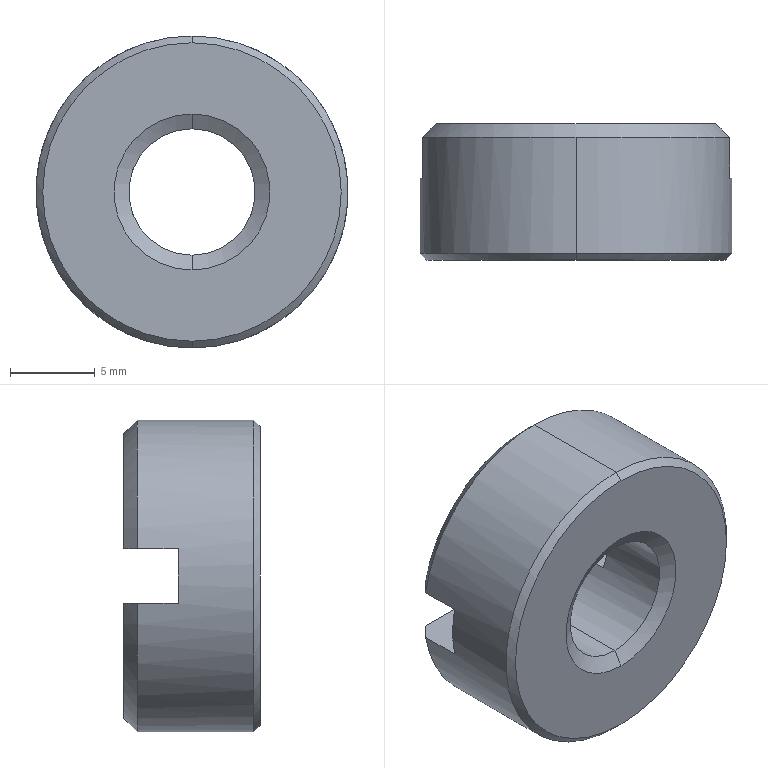Part | SolidWorks | features BaseBody 1 | 1 solid | 19 faces | box 18.462 x 8.077 x 18.462 mm | volume 1664 mm3 | plane 9 | cone 6 | cylinder 4 | commonest cylinder face diameters 7.482 x2 18.462 x2
STEP:
#1=CARTESIAN_POINT('',(66.335,375.615,109.308));
#2=VERTEX_POINT('',#1);
#3=CARTESIAN_POINT('',(57.247,375.615,116.923));
#4=VERTEX_POINT('',#3);
#5=CARTESIAN_POINT('',(57.247,375.615,107.692));
#6=DIRECTION('',(0.,-1.,0.));
#7=DIRECTION('',(0.,0.,-1.));
#8=AXIS2_PLACEMENT_3D('',#5,#6,#7);
#9=CIRCLE('',#8,9.231);
#10=EDGE_CURVE('',#2,#4,#9,.T.);
#11=ORIENTED_EDGE('',*,*,#10,.T.);
#12=CARTESIAN_POINT('',(57.247,368.75,116.923));
#13=VERTEX_POINT('',#12);
#14=CARTESIAN_POINT('',(57.247,376.423,116.923));
#15=DIRECTION('',(0.,-1.,0.));
#16=VECTOR('',#15,1000.);
#17=LINE('',#14,#16);
#18=EDGE_CURVE('',#4,#13,#17,.T.);
#19=ORIENTED_EDGE('',*,*,#18,.T.);
#20=CARTESIAN_POINT('',(57.247,368.75,98.462));
#21=VERTEX_POINT('',#20);
#22=CARTESIAN_POINT('',(57.247,368.75,107.692));
#23=DIRECTION('',(0.,1.,0.));
#24=DIRECTION('',(0.,0.,-1.));
#25=AXIS2_PLACEMENT_3D('',#22,#23,#24);
#26=CIRCLE('',#25,9.231);
#27=EDGE_CURVE('',#13,#21,#26,.T.);
#28=ORIENTED_EDGE('',*,*,#27,.T.);
#29=CARTESIAN_POINT('',(57.247,375.615,98.462));
#30=VERTEX_POINT('',#29);
#31=CARTESIAN_POINT('',(57.247,376.423,98.462));
#32=DIRECTION('',(0.,-1.,0.));
#33=VECTOR('',#32,1000.);
#34=LINE('',#31,#33);
#35=EDGE_CURVE('',#30,#21,#34,.T.);
#36=ORIENTED_EDGE('',*,*,#35,.F.);
#37=CARTESIAN_POINT('',(66.335,375.615,106.077));
#38=VERTEX_POINT('',#37);
#39=CARTESIAN_POINT('',(57.247,375.615,107.692));
#40=DIRECTION('',(0.,-1.,0.));
#41=DIRECTION('',(0.,0.,-1.));
#42=AXIS2_PLACEMENT_3D('',#39,#40,#41);
#43=CIRCLE('',#42,9.231);
#44=EDGE_CURVE('',#30,#38,#43,.T.);
#45=ORIENTED_EDGE('',*,*,#44,.T.);
#46=CARTESIAN_POINT('',(66.335,373.192,106.077));
#47=VERTEX_POINT('',#46);
#48=CARTESIAN_POINT('',(66.335,376.423,106.077));
#49=DIRECTION('',(0.,-1.,0.));
#50=VECTOR('',#49,1000.);
#51=LINE('',#48,#50);
#52=EDGE_CURVE('',#38,#47,#51,.T.);
#53=ORIENTED_EDGE('',*,*,#52,.T.);
#54=CARTESIAN_POINT('',(66.335,373.192,109.308));
#55=VERTEX_POINT('',#54);
#56=CARTESIAN_POINT('',(57.247,373.192,107.692));
#57=DIRECTION('',(0.,-1.,0.));
#58=DIRECTION('',(0.,0.,-1.));
#59=AXIS2_PLACEMENT_3D('',#56,#57,#58);
#60=CIRCLE('',#59,9.231);
#61=EDGE_CURVE('',#47,#55,#60,.T.);
#62=ORIENTED_EDGE('',*,*,#61,.T.);
#63=CARTESIAN_POINT('',(66.335,376.423,109.308));
#64=DIRECTION('',(0.,1.,0.));
#65=VECTOR('',#64,1000.);
#66=LINE('',#63,#65);
#67=EDGE_CURVE('',#55,#2,#66,.T.);
#68=ORIENTED_EDGE('',*,*,#67,.T.);
#69=EDGE_LOOP('',(#11,#19,#28,#36,#45,#53,#62,#68));
#70=FACE_OUTER_BOUND('',#69,.T.);
#71=CARTESIAN_POINT('',(57.247,376.423,107.692));
#72=DIRECTION('',(0.,-1.,0.));
#73=DIRECTION('',(0.,0.,-1.));
#74=AXIS2_PLACEMENT_3D('',#71,#72,#73);
#75=CYLINDRICAL_SURFACE('',#74,9.231);
#76=ADVANCED_FACE('',(#70),#75,.T.);
#77=CARTESIAN_POINT('',(57.247,368.346,116.519));
#78=VERTEX_POINT('',#77);
#79=CARTESIAN_POINT('',(57.247,368.346,98.865));
#80=VERTEX_POINT('',#79);
#81=CARTESIAN_POINT('',(57.247,368.346,107.692));
#82=DIRECTION('',(0.,1.,0.));
#83=DIRECTION('',(0.,0.,1.));
#84=AXIS2_PLACEMENT_3D('',#81,#82,#83);
#85=CIRCLE('',#84,8.827);
#86=EDGE_CURVE('',#78,#80,#85,.T.);
#87=ORIENTED_EDGE('',*,*,#86,.T.);
#88=CARTESIAN_POINT('',(57.247,368.75,98.462));
#89=DIRECTION('',(0.,0.7071,-0.7071));
#90=VECTOR('',#89,1000.);
#91=LINE('',#88,#90);
#92=EDGE_CURVE('',#80,#21,#91,.T.);
#93=ORIENTED_EDGE('',*,*,#92,.T.);
#94=ORIENTED_EDGE('',*,*,#27,.F.);
#95=CARTESIAN_POINT('',(57.247,368.75,116.923));
#96=DIRECTION('',(0.,0.7071,0.7071));
#97=VECTOR('',#96,1000.);
#98=LINE('',#95,#97);
#99=EDGE_CURVE('',#78,#13,#98,.T.);
#100=ORIENTED_EDGE('',*,*,#99,.F.);
#101=EDGE_LOOP('',(#87,#93,#94,#100));
#102=FACE_OUTER_BOUND('',#101,.T.);
#103=CARTESIAN_POINT('',(57.247,368.75,107.692));
#104=DIRECTION('',(0.,1.,0.));
#105=DIRECTION('',(0.,0.,1.));
#106=AXIS2_PLACEMENT_3D('',#103,#104,#105);
#107=CONICAL_SURFACE('',#106,9.231,0.7854);
#108=ADVANCED_FACE('',(#102),#107,.T.);
#109=CARTESIAN_POINT('',(57.247,376.423,111.433));
#110=VERTEX_POINT('',#109);
#111=CARTESIAN_POINT('',(53.873,376.423,109.308));
#112=VERTEX_POINT('',#111);
#113=CARTESIAN_POINT('',(57.247,376.423,107.692));
#114=DIRECTION('',(0.,-1.,0.));
#115=DIRECTION('',(0.,0.,-1.));
#116=AXIS2_PLACEMENT_3D('',#113,#114,#115);
#117=CIRCLE('',#116,3.741);
#118=EDGE_CURVE('',#110,#112,#117,.T.);
#119=ORIENTED_EDGE('',*,*,#118,.F.);
#120=CARTESIAN_POINT('',(57.247,368.851,111.433));
#121=VERTEX_POINT('',#120);
#122=CARTESIAN_POINT('',(57.247,376.423,111.433));
#123=DIRECTION('',(0.,-1.,0.));
#124=VECTOR('',#123,1000.);
#125=LINE('',#122,#124);
#126=EDGE_CURVE('',#110,#121,#125,.T.);
#127=ORIENTED_EDGE('',*,*,#126,.T.);
#128=CARTESIAN_POINT('',(57.247,368.851,103.952));
#129=VERTEX_POINT('',#128);
#130=CARTESIAN_POINT('',(57.247,368.851,107.692));
#131=DIRECTION('',(0.,1.,0.));
#132=DIRECTION('',(0.,0.,-1.));
#133=AXIS2_PLACEMENT_3D('',#130,#131,#132);
#134=CIRCLE('',#133,3.741);
#135=EDGE_CURVE('',#129,#121,#134,.T.);
#136=ORIENTED_EDGE('',*,*,#135,.F.);
#137=CARTESIAN_POINT('',(57.247,376.423,103.952));
#138=VERTEX_POINT('',#137);
#139=CARTESIAN_POINT('',(57.247,376.423,103.952));
#140=DIRECTION('',(0.,-1.,0.));
#141=VECTOR('',#140,1000.);
#142=LINE('',#139,#141);
#143=EDGE_CURVE('',#138,#129,#142,.T.);
#144=ORIENTED_EDGE('',*,*,#143,.F.);
#145=CARTESIAN_POINT('',(53.873,376.423,106.077));
#146=VERTEX_POINT('',#145);
#147=CARTESIAN_POINT('',(57.247,376.423,107.692));
#148=DIRECTION('',(0.,1.,0.));
#149=DIRECTION('',(0.,0.,-1.));
#150=AXIS2_PLACEMENT_3D('',#147,#148,#149);
#151=CIRCLE('',#150,3.741);
#152=EDGE_CURVE('',#138,#146,#151,.T.);
#153=ORIENTED_EDGE('',*,*,#152,.T.);
#154=CARTESIAN_POINT('',(53.873,373.192,106.077));
#155=VERTEX_POINT('',#154);
#156=CARTESIAN_POINT('',(53.873,381.269,106.077));
#157=DIRECTION('',(0.,1.,0.));
#158=VECTOR('',#157,1000.);
#159=LINE('',#156,#158);
#160=EDGE_CURVE('',#155,#146,#159,.T.);
#161=ORIENTED_EDGE('',*,*,#160,.F.);
#162=CARTESIAN_POINT('',(53.873,373.192,109.308));
#163=VERTEX_POINT('',#162);
#164=CARTESIAN_POINT('',(57.247,373.192,107.692));
#165=DIRECTION('',(0.,-1.,0.));
#166=DIRECTION('',(0.,0.,-1.));
#167=AXIS2_PLACEMENT_3D('',#164,#165,#166);
#168=CIRCLE('',#167,3.741);
#169=EDGE_CURVE('',#163,#155,#168,.T.);
#170=ORIENTED_EDGE('',*,*,#169,.F.);
#171=CARTESIAN_POINT('',(53.873,373.192,109.308));
#172=DIRECTION('',(0.,-1.,0.));
#173=VECTOR('',#172,1000.);
#174=LINE('',#171,#173);
#175=EDGE_CURVE('',#112,#163,#174,.T.);
#176=ORIENTED_EDGE('',*,*,#175,.F.);
#177=EDGE_LOOP('',(#119,#127,#136,#144,#153,#161,#170,#176));
#178=FACE_OUTER_BOUND('',#177,.T.);
#179=CARTESIAN_POINT('',(57.247,376.423,107.692));
#180=DIRECTION('',(0.,-1.,0.));
#181=DIRECTION('',(0.,0.,-1.));
#182=AXIS2_PLACEMENT_3D('',#179,#180,#181);
#183=CYLINDRICAL_SURFACE('',#182,3.741);
#184=ADVANCED_FACE('',(#178),#183,.F.);
#185=ORIENTED_EDGE('',*,*,#135,.T.);
#186=CARTESIAN_POINT('',(57.247,368.346,112.308));
#187=VERTEX_POINT('',#186);
#188=CARTESIAN_POINT('',(57.247,368.346,112.308));
#189=DIRECTION('',(0.,-0.5,0.866));
#190=VECTOR('',#189,1000.);
#191=LINE('',#188,#190);
#192=EDGE_CURVE('',#121,#187,#191,.T.);
#193=ORIENTED_EDGE('',*,*,#192,.T.);
#194=CARTESIAN_POINT('',(57.247,368.346,103.077));
#195=VERTEX_POINT('',#194);
#196=CARTESIAN_POINT('',(57.247,368.346,107.692));
#197=DIRECTION('',(0.,-1.,0.));
#198=DIRECTION('',(0.,0.,-1.));
#199=AXIS2_PLACEMENT_3D('',#196,#197,#198);
#200=CIRCLE('',#199,4.615);
#201=EDGE_CURVE('',#187,#195,#200,.T.);
#202=ORIENTED_EDGE('',*,*,#201,.T.);
#203=CARTESIAN_POINT('',(57.247,368.346,103.077));
#204=DIRECTION('',(0.,-0.5,-0.866));
#205=VECTOR('',#204,1000.);
#206=LINE('',#203,#205);
#207=EDGE_CURVE('',#129,#195,#206,.T.);
#208=ORIENTED_EDGE('',*,*,#207,.F.);
#209=EDGE_LOOP('',(#185,#193,#202,#208));
#210=FACE_OUTER_BOUND('',#209,.T.);
#211=CARTESIAN_POINT('',(57.247,368.346,107.692));
#212=DIRECTION('',(0.,-1.,0.));
#213=DIRECTION('',(0.,0.,-1.));
#214=AXIS2_PLACEMENT_3D('',#211,#212,#213);
#215=CONICAL_SURFACE('',#214,4.615,1.047);
#216=ADVANCED_FACE('',(#210),#215,.F.);
#217=ORIENTED_EDGE('',*,*,#18,.F.);
#218=CARTESIAN_POINT('',(48.158,375.615,109.308));
#219=VERTEX_POINT('',#218);
#220=CARTESIAN_POINT('',(57.247,375.615,107.692));
#221=DIRECTION('',(0.,-1.,0.));
#222=DIRECTION('',(0.,0.,-1.));
#223=AXIS2_PLACEMENT_3D('',#220,#221,#222);
#224=CIRCLE('',#223,9.231);
#225=EDGE_CURVE('',#4,#219,#224,.T.);
#226=ORIENTED_EDGE('',*,*,#225,.T.);
#227=CARTESIAN_POINT('',(48.158,373.192,109.308));
#228=VERTEX_POINT('',#227);
#229=CARTESIAN_POINT('',(48.158,376.423,109.308));
#230=DIRECTION('',(0.,-1.,0.));
#231=VECTOR('',#230,1000.);
#232=LINE('',#229,#231);
#233=EDGE_CURVE('',#219,#228,#232,.T.);
#234=ORIENTED_EDGE('',*,*,#233,.T.);
#235=CARTESIAN_POINT('',(48.158,373.192,106.077));
#236=VERTEX_POINT('',#235);
#237=CARTESIAN_POINT('',(57.247,373.192,107.692));
#238=DIRECTION('',(0.,-1.,0.));
#239=DIRECTION('',(0.,0.,-1.));
#240=AXIS2_PLACEMENT_3D('',#237,#238,#239);
#241=CIRCLE('',#240,9.231);
#242=EDGE_CURVE('',#228,#236,#241,.T.);
#243=ORIENTED_EDGE('',*,*,#242,.T.);
#244=CARTESIAN_POINT('',(48.158,375.615,106.077));
#245=VERTEX_POINT('',#244);
#246=CARTESIAN_POINT('',(48.158,376.423,106.077));
#247=DIRECTION('',(0.,1.,0.));
#248=VECTOR('',#247,1000.);
#249=LINE('',#246,#248);
#250=EDGE_CURVE('',#236,#245,#249,.T.);
#251=ORIENTED_EDGE('',*,*,#250,.T.);
#252=CARTESIAN_POINT('',(57.247,375.615,107.692));
#253=DIRECTION('',(0.,-1.,0.));
#254=DIRECTION('',(0.,0.,-1.));
#255=AXIS2_PLACEMENT_3D('',#252,#253,#254);
#256=CIRCLE('',#255,9.231);
#257=EDGE_CURVE('',#245,#30,#256,.T.);
#258=ORIENTED_EDGE('',*,*,#257,.T.);
#259=ORIENTED_EDGE('',*,*,#35,.T.);
#260=CARTESIAN_POINT('',(57.247,368.75,107.692));
#261=DIRECTION('',(0.,1.,0.));
#262=DIRECTION('',(0.,0.,-1.));
#263=AXIS2_PLACEMENT_3D('',#260,#261,#262);
#264=CIRCLE('',#263,9.231);
#265=EDGE_CURVE('',#21,#13,#264,.T.);
#266=ORIENTED_EDGE('',*,*,#265,.T.);
#267=EDGE_LOOP('',(#217,#226,#234,#243,#251,#258,#259,#266));
#268=FACE_OUTER_BOUND('',#267,.T.);
#269=CARTESIAN_POINT('',(57.247,376.423,107.692));
#270=DIRECTION('',(0.,-1.,0.));
#271=DIRECTION('',(0.,0.,-1.));
#272=AXIS2_PLACEMENT_3D('',#269,#270,#271);
#273=CYLINDRICAL_SURFACE('',#272,9.231);
#274=ADVANCED_FACE('',(#268),#273,.T.);
#275=ORIENTED_EDGE('',*,*,#257,.F.);
#276=CARTESIAN_POINT('',(48.98,376.423,106.077));
#277=VERTEX_POINT('',#276);
#278=CARTESIAN_POINT('',(48.158,375.615,106.077));
#279=CARTESIAN_POINT('',(48.432,375.885,106.077));
#280=CARTESIAN_POINT('',(48.706,376.154,106.077));
#281=CARTESIAN_POINT('',(48.98,376.423,106.077));
#282=B_SPLINE_CURVE_WITH_KNOTS('',3,(#278,#279,#280,#281),.UNSPECIFIED.,.F.,.F.,(4,4),(0.,0.001152),.UNSPECIFIED.);
#283=EDGE_CURVE('',#245,#277,#282,.T.);
#284=ORIENTED_EDGE('',*,*,#283,.T.);
#285=CARTESIAN_POINT('',(65.513,376.423,106.077));
#286=VERTEX_POINT('',#285);
#287=CARTESIAN_POINT('',(57.247,376.423,107.692));
#288=DIRECTION('',(0.,-1.,0.));
#289=DIRECTION('',(1.,0.,0.));
#290=AXIS2_PLACEMENT_3D('',#287,#288,#289);
#291=CIRCLE('',#290,8.423);
#292=EDGE_CURVE('',#277,#286,#291,.T.);
#293=ORIENTED_EDGE('',*,*,#292,.T.);
#294=CARTESIAN_POINT('',(65.513,376.423,106.077));
#295=CARTESIAN_POINT('',(65.787,376.154,106.077));
#296=CARTESIAN_POINT('',(66.061,375.885,106.077));
#297=CARTESIAN_POINT('',(66.335,375.615,106.077));
#298=B_SPLINE_CURVE_WITH_KNOTS('',3,(#294,#295,#296,#297),.UNSPECIFIED.,.F.,.F.,(4,4),(0.,0.001152),.UNSPECIFIED.);
#299=EDGE_CURVE('',#286,#38,#298,.T.);
#300=ORIENTED_EDGE('',*,*,#299,.T.);
#301=ORIENTED_EDGE('',*,*,#44,.F.);
#302=EDGE_LOOP('',(#275,#284,#293,#300,#301));
#303=FACE_OUTER_BOUND('',#302,.T.);
#304=CARTESIAN_POINT('',(57.247,375.615,107.692));
#305=DIRECTION('',(0.,-1.,0.));
#306=DIRECTION('',(1.,0.,0.));
#307=AXIS2_PLACEMENT_3D('',#304,#305,#306);
#308=CONICAL_SURFACE('',#307,9.231,0.7854);
#309=ADVANCED_FACE('',(#303),#308,.T.);
#310=ORIENTED_EDGE('',*,*,#160,.T.);
#311=CARTESIAN_POINT('',(38.785,376.423,106.077));
#312=DIRECTION('',(-1.,0.,0.));
#313=VECTOR('',#312,1000.);
#314=LINE('',#311,#313);
#315=EDGE_CURVE('',#146,#277,#314,.T.);
#316=ORIENTED_EDGE('',*,*,#315,.T.);
#317=ORIENTED_EDGE('',*,*,#283,.F.);
#318=ORIENTED_EDGE('',*,*,#250,.F.);
#319=CARTESIAN_POINT('',(38.785,373.192,106.077));
#320=DIRECTION('',(1.,0.,0.));
#321=VECTOR('',#320,1000.);
#322=LINE('',#319,#321);
#323=EDGE_CURVE('',#236,#155,#322,.T.);
#324=ORIENTED_EDGE('',*,*,#323,.T.);
#325=EDGE_LOOP('',(#310,#316,#317,#318,#324));
#326=FACE_OUTER_BOUND('',#325,.T.);
#327=CARTESIAN_POINT('',(38.785,381.269,106.077));
#328=DIRECTION('',(0.,0.,1.));
#329=DIRECTION('',(1.,0.,0.));
#330=AXIS2_PLACEMENT_3D('',#327,#328,#329);
#331=PLANE('',#330);
#332=ADVANCED_FACE('',(#326),#331,.T.);
#333=CARTESIAN_POINT('',(38.785,373.192,109.308));
#334=DIRECTION('',(1.,0.,0.));
#335=VECTOR('',#334,1000.);
#336=LINE('',#333,#335);
#337=EDGE_CURVE('',#228,#163,#336,.T.);
#338=ORIENTED_EDGE('',*,*,#337,.T.);
#339=ORIENTED_EDGE('',*,*,#169,.T.);
#340=ORIENTED_EDGE('',*,*,#323,.F.);
#341=ORIENTED_EDGE('',*,*,#242,.F.);
#342=EDGE_LOOP('',(#338,#339,#340,#341));
#343=FACE_OUTER_BOUND('',#342,.T.);
#344=CARTESIAN_POINT('',(38.785,373.192,106.077));
#345=DIRECTION('',(0.,1.,0.));
#346=DIRECTION('',(0.,0.,1.));
#347=AXIS2_PLACEMENT_3D('',#344,#345,#346);
#348=PLANE('',#347);
#349=ADVANCED_FACE('',(#343),#348,.T.);
#350=CARTESIAN_POINT('',(48.98,376.423,109.308));
#351=VERTEX_POINT('',#350);
#352=CARTESIAN_POINT('',(38.785,376.423,109.308));
#353=DIRECTION('',(1.,0.,0.));
#354=VECTOR('',#353,1000.);
#355=LINE('',#352,#354);
#356=EDGE_CURVE('',#351,#112,#355,.T.);
#357=ORIENTED_EDGE('',*,*,#356,.T.);
#358=ORIENTED_EDGE('',*,*,#175,.T.);
#359=ORIENTED_EDGE('',*,*,#337,.F.);
#360=ORIENTED_EDGE('',*,*,#233,.F.);
#361=CARTESIAN_POINT('',(48.158,375.615,109.308));
#362=CARTESIAN_POINT('',(48.432,375.885,109.308));
#363=CARTESIAN_POINT('',(48.706,376.154,109.308));
#364=CARTESIAN_POINT('',(48.98,376.423,109.308));
#365=B_SPLINE_CURVE_WITH_KNOTS('',3,(#361,#362,#363,#364),.UNSPECIFIED.,.F.,.F.,(4,4),(0.,0.001152),.UNSPECIFIED.);
#366=EDGE_CURVE('',#219,#351,#365,.T.);
#367=ORIENTED_EDGE('',*,*,#366,.T.);
#368=EDGE_LOOP('',(#357,#358,#359,#360,#367));
#369=FACE_OUTER_BOUND('',#368,.T.);
#370=CARTESIAN_POINT('',(38.785,373.192,109.308));
#371=DIRECTION('',(0.,0.,-1.));
#372=DIRECTION('',(-1.,0.,0.));
#373=AXIS2_PLACEMENT_3D('',#370,#371,#372);
#374=PLANE('',#373);
#375=ADVANCED_FACE('',(#369),#374,.T.);
#376=ORIENTED_EDGE('',*,*,#10,.F.);
#377=CARTESIAN_POINT('',(65.513,376.423,109.308));
#378=VERTEX_POINT('',#377);
#379=CARTESIAN_POINT('',(66.335,375.615,109.308));
#380=CARTESIAN_POINT('',(66.061,375.885,109.308));
#381=CARTESIAN_POINT('',(65.787,376.154,109.308));
#382=CARTESIAN_POINT('',(65.513,376.423,109.308));
#383=B_SPLINE_CURVE_WITH_KNOTS('',3,(#379,#380,#381,#382),.UNSPECIFIED.,.F.,.F.,(4,4),(0.,0.001152),.UNSPECIFIED.);
#384=EDGE_CURVE('',#2,#378,#383,.T.);
#385=ORIENTED_EDGE('',*,*,#384,.T.);
#386=CARTESIAN_POINT('',(57.247,376.423,107.692));
#387=DIRECTION('',(0.,-1.,0.));
#388=DIRECTION('',(0.,0.,-1.));
#389=AXIS2_PLACEMENT_3D('',#386,#387,#388);
#390=CIRCLE('',#389,8.423);
#391=EDGE_CURVE('',#378,#351,#390,.T.);
#392=ORIENTED_EDGE('',*,*,#391,.T.);
#393=ORIENTED_EDGE('',*,*,#366,.F.);
#394=ORIENTED_EDGE('',*,*,#225,.F.);
#395=EDGE_LOOP('',(#376,#385,#392,#393,#394));
#396=FACE_OUTER_BOUND('',#395,.T.);
#397=CARTESIAN_POINT('',(57.247,375.615,107.692));
#398=DIRECTION('',(0.,-1.,0.));
#399=DIRECTION('',(0.,0.,-1.));
#400=AXIS2_PLACEMENT_3D('',#397,#398,#399);
#401=CONICAL_SURFACE('',#400,9.231,0.7854);
#402=ADVANCED_FACE('',(#396),#401,.T.);
#403=ORIENTED_EDGE('',*,*,#92,.F.);
#404=CARTESIAN_POINT('',(57.247,368.346,107.692));
#405=DIRECTION('',(0.,1.,0.));
#406=DIRECTION('',(0.,0.,1.));
#407=AXIS2_PLACEMENT_3D('',#404,#405,#406);
#408=CIRCLE('',#407,8.827);
#409=EDGE_CURVE('',#80,#78,#408,.T.);
#410=ORIENTED_EDGE('',*,*,#409,.T.);
#411=ORIENTED_EDGE('',*,*,#99,.T.);
#412=ORIENTED_EDGE('',*,*,#265,.F.);
#413=EDGE_LOOP('',(#403,#410,#411,#412));
#414=FACE_OUTER_BOUND('',#413,.T.);
#415=CARTESIAN_POINT('',(57.247,368.75,107.692));
#416=DIRECTION('',(0.,1.,0.));
#417=DIRECTION('',(0.,0.,1.));
#418=AXIS2_PLACEMENT_3D('',#415,#416,#417);
#419=CONICAL_SURFACE('',#418,9.231,0.7854);
#420=ADVANCED_FACE('',(#414),#419,.T.);
#421=CARTESIAN_POINT('',(60.621,376.423,106.077));
#422=VERTEX_POINT('',#421);
#423=CARTESIAN_POINT('',(38.785,376.423,106.077));
#424=DIRECTION('',(-1.,0.,0.));
#425=VECTOR('',#424,1000.);
#426=LINE('',#423,#425);
#427=EDGE_CURVE('',#286,#422,#426,.T.);
#428=ORIENTED_EDGE('',*,*,#427,.T.);
#429=CARTESIAN_POINT('',(60.621,373.192,106.077));
#430=VERTEX_POINT('',#429);
#431=CARTESIAN_POINT('',(60.621,381.269,106.077));
#432=DIRECTION('',(0.,-1.,0.));
#433=VECTOR('',#432,1000.);
#434=LINE('',#431,#433);
#435=EDGE_CURVE('',#422,#430,#434,.T.);
#436=ORIENTED_EDGE('',*,*,#435,.T.);
#437=CARTESIAN_POINT('',(38.785,373.192,106.077));
#438=DIRECTION('',(1.,0.,0.));
#439=VECTOR('',#438,1000.);
#440=LINE('',#437,#439);
#441=EDGE_CURVE('',#430,#47,#440,.T.);
#442=ORIENTED_EDGE('',*,*,#441,.T.);
#443=ORIENTED_EDGE('',*,*,#52,.F.);
#444=ORIENTED_EDGE('',*,*,#299,.F.);
#445=EDGE_LOOP('',(#428,#436,#442,#443,#444));
#446=FACE_OUTER_BOUND('',#445,.T.);
#447=CARTESIAN_POINT('',(38.785,381.269,106.077));
#448=DIRECTION('',(0.,0.,1.));
#449=DIRECTION('',(1.,0.,0.));
#450=AXIS2_PLACEMENT_3D('',#447,#448,#449);
#451=PLANE('',#450);
#452=ADVANCED_FACE('',(#446),#451,.T.);
#453=ORIENTED_EDGE('',*,*,#315,.F.);
#454=ORIENTED_EDGE('',*,*,#152,.F.);
#455=CARTESIAN_POINT('',(57.247,376.423,107.692));
#456=DIRECTION('',(0.,1.,0.));
#457=DIRECTION('',(0.,0.,-1.));
#458=AXIS2_PLACEMENT_3D('',#455,#456,#457);
#459=CIRCLE('',#458,3.741);
#460=EDGE_CURVE('',#422,#138,#459,.T.);
#461=ORIENTED_EDGE('',*,*,#460,.F.);
#462=ORIENTED_EDGE('',*,*,#427,.F.);
#463=ORIENTED_EDGE('',*,*,#292,.F.);
#464=EDGE_LOOP('',(#453,#454,#461,#462,#463));
#465=FACE_OUTER_BOUND('',#464,.T.);
#466=CARTESIAN_POINT('',(48.823,376.423,107.692));
#467=DIRECTION('',(0.,-1.,0.));
#468=DIRECTION('',(0.,0.,-1.));
#469=AXIS2_PLACEMENT_3D('',#466,#467,#468);
#470=PLANE('',#469);
#471=ADVANCED_FACE('',(#465),#470,.F.);
#472=ORIENTED_EDGE('',*,*,#126,.F.);
#473=CARTESIAN_POINT('',(60.621,376.423,109.308));
#474=VERTEX_POINT('',#473);
#475=CARTESIAN_POINT('',(57.247,376.423,107.692));
#476=DIRECTION('',(0.,-1.,0.));
#477=DIRECTION('',(0.,0.,-1.));
#478=AXIS2_PLACEMENT_3D('',#475,#476,#477);
#479=CIRCLE('',#478,3.741);
#480=EDGE_CURVE('',#474,#110,#479,.T.);
#481=ORIENTED_EDGE('',*,*,#480,.F.);
#482=CARTESIAN_POINT('',(60.621,373.192,109.308));
#483=VERTEX_POINT('',#482);
#484=CARTESIAN_POINT('',(60.621,373.192,109.308));
#485=DIRECTION('',(0.,1.,0.));
#486=VECTOR('',#485,1000.);
#487=LINE('',#484,#486);
#488=EDGE_CURVE('',#483,#474,#487,.T.);
#489=ORIENTED_EDGE('',*,*,#488,.F.);
#490=CARTESIAN_POINT('',(57.247,373.192,107.692));
#491=DIRECTION('',(0.,-1.,0.));
#492=DIRECTION('',(0.,0.,-1.));
#493=AXIS2_PLACEMENT_3D('',#490,#491,#492);
#494=CIRCLE('',#493,3.741);
#495=EDGE_CURVE('',#430,#483,#494,.T.);
#496=ORIENTED_EDGE('',*,*,#495,.F.);
#497=ORIENTED_EDGE('',*,*,#435,.F.);
#498=ORIENTED_EDGE('',*,*,#460,.T.);
#499=ORIENTED_EDGE('',*,*,#143,.T.);
#500=CARTESIAN_POINT('',(57.247,368.851,107.692));
#501=DIRECTION('',(0.,1.,0.));
#502=DIRECTION('',(0.,0.,-1.));
#503=AXIS2_PLACEMENT_3D('',#500,#501,#502);
#504=CIRCLE('',#503,3.741);
#505=EDGE_CURVE('',#121,#129,#504,.T.);
#506=ORIENTED_EDGE('',*,*,#505,.F.);
#507=EDGE_LOOP('',(#472,#481,#489,#496,#497,#498,#499,#506));
#508=FACE_OUTER_BOUND('',#507,.T.);
#509=CARTESIAN_POINT('',(57.247,376.423,107.692));
#510=DIRECTION('',(0.,-1.,0.));
#511=DIRECTION('',(0.,0.,-1.));
#512=AXIS2_PLACEMENT_3D('',#509,#510,#511);
#513=CYLINDRICAL_SURFACE('',#512,3.741);
#514=ADVANCED_FACE('',(#508),#513,.F.);
#515=CARTESIAN_POINT('',(48.823,376.423,109.308));
#516=DIRECTION('',(1.,0.,0.));
#517=VECTOR('',#516,1000.);
#518=LINE('',#515,#517);
#519=EDGE_CURVE('',#474,#378,#518,.T.);
#520=ORIENTED_EDGE('',*,*,#519,.F.);
#521=ORIENTED_EDGE('',*,*,#480,.T.);
#522=ORIENTED_EDGE('',*,*,#118,.T.);
#523=ORIENTED_EDGE('',*,*,#356,.F.);
#524=ORIENTED_EDGE('',*,*,#391,.F.);
#525=EDGE_LOOP('',(#520,#521,#522,#523,#524));
#526=FACE_OUTER_BOUND('',#525,.T.);
#527=CARTESIAN_POINT('',(48.823,376.423,107.692));
#528=DIRECTION('',(0.,-1.,0.));
#529=DIRECTION('',(0.,0.,-1.));
#530=AXIS2_PLACEMENT_3D('',#527,#528,#529);
#531=PLANE('',#530);
#532=ADVANCED_FACE('',(#526),#531,.F.);
#533=ORIENTED_EDGE('',*,*,#488,.T.);
#534=ORIENTED_EDGE('',*,*,#519,.T.);
#535=ORIENTED_EDGE('',*,*,#384,.F.);
#536=ORIENTED_EDGE('',*,*,#67,.F.);
#537=CARTESIAN_POINT('',(38.785,373.192,109.308));
#538=DIRECTION('',(-1.,0.,0.));
#539=VECTOR('',#538,1000.);
#540=LINE('',#537,#539);
#541=EDGE_CURVE('',#55,#483,#540,.T.);
#542=ORIENTED_EDGE('',*,*,#541,.T.);
#543=EDGE_LOOP('',(#533,#534,#535,#536,#542));
#544=FACE_OUTER_BOUND('',#543,.T.);
#545=CARTESIAN_POINT('',(38.785,373.192,109.308));
#546=DIRECTION('',(0.,0.,-1.));
#547=DIRECTION('',(-1.,0.,0.));
#548=AXIS2_PLACEMENT_3D('',#545,#546,#547);
#549=PLANE('',#548);
#550=ADVANCED_FACE('',(#544),#549,.T.);
#551=ORIENTED_EDGE('',*,*,#441,.F.);
#552=ORIENTED_EDGE('',*,*,#495,.T.);
#553=ORIENTED_EDGE('',*,*,#541,.F.);
#554=ORIENTED_EDGE('',*,*,#61,.F.);
#555=EDGE_LOOP('',(#551,#552,#553,#554));
#556=FACE_OUTER_BOUND('',#555,.T.);
#557=CARTESIAN_POINT('',(38.785,373.192,106.077));
#558=DIRECTION('',(0.,1.,0.));
#559=DIRECTION('',(0.,0.,1.));
#560=AXIS2_PLACEMENT_3D('',#557,#558,#559);
#561=PLANE('',#560);
#562=ADVANCED_FACE('',(#556),#561,.T.);
#563=CARTESIAN_POINT('',(57.247,368.346,107.692));
#564=DIRECTION('',(0.,-1.,0.));
#565=DIRECTION('',(0.,0.,-1.));
#566=AXIS2_PLACEMENT_3D('',#563,#564,#565);
#567=CIRCLE('',#566,4.615);
#568=EDGE_CURVE('',#195,#187,#567,.T.);
#569=ORIENTED_EDGE('',*,*,#568,.F.);
#570=ORIENTED_EDGE('',*,*,#201,.F.);
#571=EDGE_LOOP('',(#569,#570));
#572=FACE_BOUND('',#571,.T.);
#573=ORIENTED_EDGE('',*,*,#86,.F.);
#574=ORIENTED_EDGE('',*,*,#409,.F.);
#575=EDGE_LOOP('',(#573,#574));
#576=FACE_OUTER_BOUND('',#575,.T.);
#577=CARTESIAN_POINT('',(57.247,368.346,107.692));
#578=DIRECTION('',(0.,1.,0.));
#579=DIRECTION('',(0.,0.,1.));
#580=AXIS2_PLACEMENT_3D('',#577,#578,#579);
#581=PLANE('',#580);
#582=ADVANCED_FACE('',(#572,#576),#581,.F.);
#583=ORIENTED_EDGE('',*,*,#192,.F.);
#584=ORIENTED_EDGE('',*,*,#505,.T.);
#585=ORIENTED_EDGE('',*,*,#207,.T.);
#586=ORIENTED_EDGE('',*,*,#568,.T.);
#587=EDGE_LOOP('',(#583,#584,#585,#586));
#588=FACE_OUTER_BOUND('',#587,.T.);
#589=CARTESIAN_POINT('',(57.247,368.346,107.692));
#590=DIRECTION('',(0.,-1.,0.));
#591=DIRECTION('',(0.,0.,-1.));
#592=AXIS2_PLACEMENT_3D('',#589,#590,#591);
#593=CONICAL_SURFACE('',#592,4.615,1.047);
#594=ADVANCED_FACE('',(#588),#593,.F.);
#595=CLOSED_SHELL('',(#76,#108,#184,#216,#274,#309,#332,#349,#375,#402,#420,#452,#471,#514,#532,#550,#562,#582,#594));
#596=MANIFOLD_SOLID_BREP('',#595);
#597=CARTESIAN_POINT('',(0.,0.,0.));
#598=DIRECTION('',(0.,0.,1.));
#599=DIRECTION('',(1.,0.,0.));
#600=AXIS2_PLACEMENT_3D('',#597,#598,#599);
#601=(LENGTH_UNIT()NAMED_UNIT(*)SI_UNIT(.MILLI.,.METRE.));
#602=UNCERTAINTY_MEASURE_WITH_UNIT(LENGTH_MEASURE(0.00001),#601,'','');
#603=(NAMED_UNIT(*)PLANE_ANGLE_UNIT()SI_UNIT($,.RADIAN.));
#604=(NAMED_UNIT(*)SI_UNIT($,.STERADIAN.)SOLID_ANGLE_UNIT());
#605=(GEOMETRIC_REPRESENTATION_CONTEXT(3)GLOBAL_UNCERTAINTY_ASSIGNED_CONTEXT((#602))GLOBAL_UNIT_ASSIGNED_CONTEXT((#601,#603,#604))REPRESENTATION_CONTEXT('',''));
#606=ADVANCED_BREP_SHAPE_REPRESENTATION('',(#596,#600),#605);